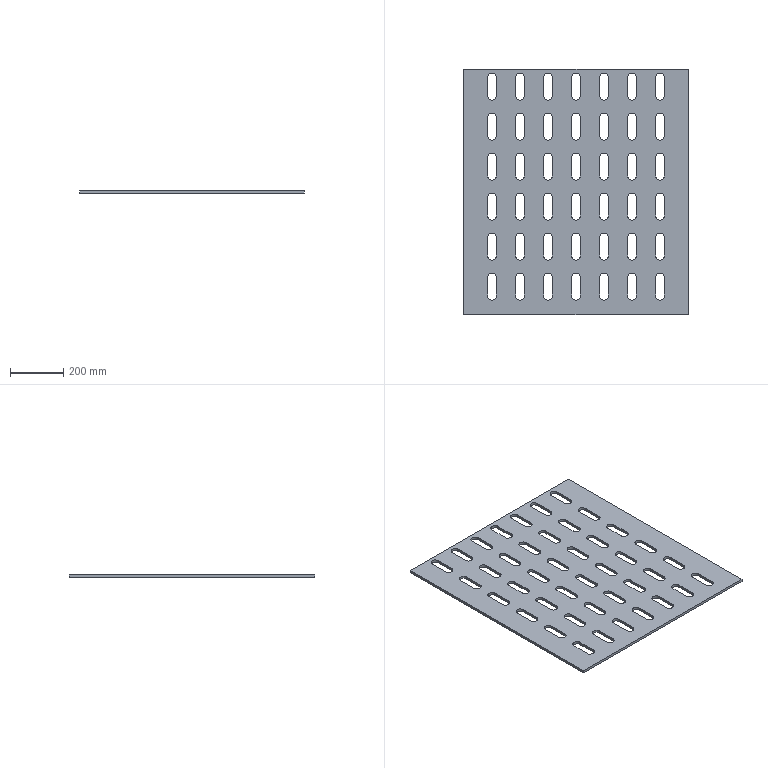Part | SolidWorks | features Extrusion 1, ICE 1 | 1 solid | 174 faces | box 840 x 920 x 10 mm | volume 6461489 mm3 | plane 90 | cylinder 84 | commonest cylinder face diameters 31.761 x84